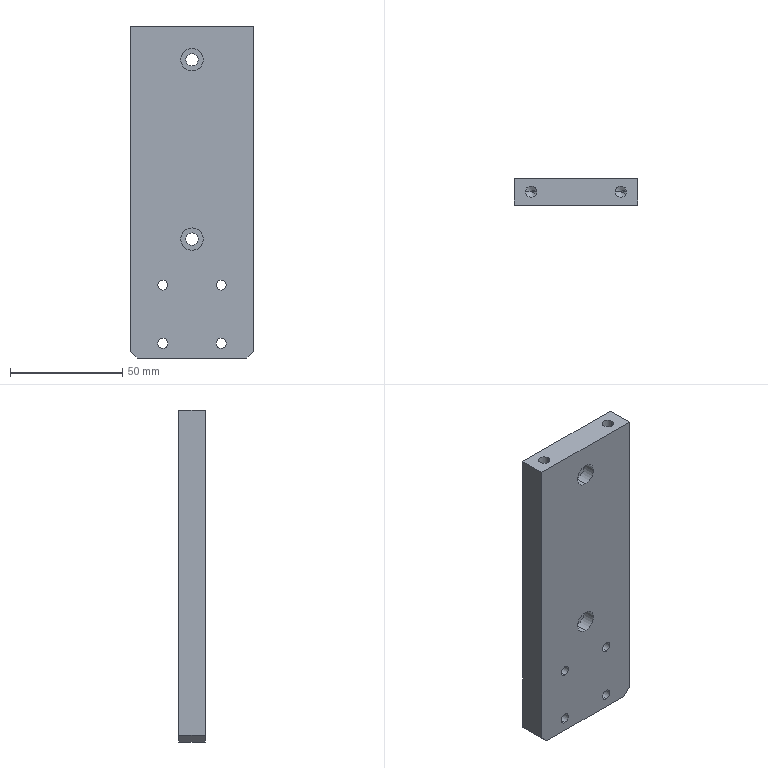Part | SolidWorks | features HoleWzd 3, Chamfer 1, Extrusion 1 | 1 solid | 46 faces | box 55 x 12 x 148 mm | volume 94373 mm3 | cylinder 28 | plane 14 | cone 4 | commonest cylinder face diameters 4.5 x8 8 x8 5 x4 5.5 x4 10 x4
STEP:
#1=CARTESIAN_POINT('',(0.,-0.3,64.));
#2=VERTEX_POINT('',#1);
#3=CARTESIAN_POINT('',(0.,-0.3,54.));
#4=VERTEX_POINT('',#3);
#5=CARTESIAN_POINT('',(0.,-0.3,59.));
#6=DIRECTION('',(0.,-1.,0.));
#7=DIRECTION('',(0.,0.,-1.));
#8=AXIS2_PLACEMENT_3D('',#5,#6,#7);
#9=CIRCLE('',#8,5.);
#10=EDGE_CURVE('',#2,#4,#9,.T.);
#11=ORIENTED_EDGE('',*,*,#10,.F.);
#12=CARTESIAN_POINT('',(0.,-6.,64.));
#13=VERTEX_POINT('',#12);
#14=CARTESIAN_POINT('',(0.,-6.,64.));
#15=DIRECTION('',(0.,-1.,0.));
#16=VECTOR('',#15,1000.);
#17=LINE('',#14,#16);
#18=EDGE_CURVE('',#2,#13,#17,.T.);
#19=ORIENTED_EDGE('',*,*,#18,.T.);
#20=CARTESIAN_POINT('',(0.,-6.,54.));
#21=VERTEX_POINT('',#20);
#22=CARTESIAN_POINT('',(0.,-6.,59.));
#23=DIRECTION('',(0.,-1.,0.));
#24=DIRECTION('',(0.,0.,-1.));
#25=AXIS2_PLACEMENT_3D('',#22,#23,#24);
#26=CIRCLE('',#25,5.);
#27=EDGE_CURVE('',#13,#21,#26,.T.);
#28=ORIENTED_EDGE('',*,*,#27,.T.);
#29=CARTESIAN_POINT('',(0.,-6.,54.));
#30=DIRECTION('',(0.,-1.,0.));
#31=VECTOR('',#30,1000.);
#32=LINE('',#29,#31);
#33=EDGE_CURVE('',#4,#21,#32,.T.);
#34=ORIENTED_EDGE('',*,*,#33,.F.);
#35=EDGE_LOOP('',(#11,#19,#28,#34));
#36=FACE_OUTER_BOUND('',#35,.T.);
#37=CARTESIAN_POINT('',(0.,-6.,59.));
#38=DIRECTION('',(0.,-1.,0.));
#39=DIRECTION('',(0.,0.,-1.));
#40=AXIS2_PLACEMENT_3D('',#37,#38,#39);
#41=CYLINDRICAL_SURFACE('',#40,5.);
#42=ADVANCED_FACE('',(#36),#41,.F.);
#43=CARTESIAN_POINT('',(0.,6.,61.75));
#44=VERTEX_POINT('',#43);
#45=CARTESIAN_POINT('',(0.,6.,56.25));
#46=VERTEX_POINT('',#45);
#47=CARTESIAN_POINT('',(0.,6.,59.));
#48=DIRECTION('',(0.,-1.,0.));
#49=DIRECTION('',(0.,0.,-1.));
#50=AXIS2_PLACEMENT_3D('',#47,#48,#49);
#51=CIRCLE('',#50,2.75);
#52=EDGE_CURVE('',#44,#46,#51,.T.);
#53=ORIENTED_EDGE('',*,*,#52,.F.);
#54=CARTESIAN_POINT('',(0.,-0.3,61.75));
#55=VERTEX_POINT('',#54);
#56=CARTESIAN_POINT('',(0.,-6.,61.75));
#57=DIRECTION('',(0.,-1.,0.));
#58=VECTOR('',#57,1000.);
#59=LINE('',#56,#58);
#60=EDGE_CURVE('',#44,#55,#59,.T.);
#61=ORIENTED_EDGE('',*,*,#60,.T.);
#62=CARTESIAN_POINT('',(0.,-0.3,56.25));
#63=VERTEX_POINT('',#62);
#64=CARTESIAN_POINT('',(0.,-0.3,59.));
#65=DIRECTION('',(0.,-1.,0.));
#66=DIRECTION('',(0.,0.,-1.));
#67=AXIS2_PLACEMENT_3D('',#64,#65,#66);
#68=CIRCLE('',#67,2.75);
#69=EDGE_CURVE('',#55,#63,#68,.T.);
#70=ORIENTED_EDGE('',*,*,#69,.T.);
#71=CARTESIAN_POINT('',(0.,-6.,56.25));
#72=DIRECTION('',(0.,-1.,0.));
#73=VECTOR('',#72,1000.);
#74=LINE('',#71,#73);
#75=EDGE_CURVE('',#46,#63,#74,.T.);
#76=ORIENTED_EDGE('',*,*,#75,.F.);
#77=EDGE_LOOP('',(#53,#61,#70,#76));
#78=FACE_OUTER_BOUND('',#77,.T.);
#79=CARTESIAN_POINT('',(0.,-6.,59.));
#80=DIRECTION('',(0.,-1.,0.));
#81=DIRECTION('',(0.,0.,-1.));
#82=AXIS2_PLACEMENT_3D('',#79,#80,#81);
#83=CYLINDRICAL_SURFACE('',#82,2.75);
#84=ADVANCED_FACE('',(#78),#83,.F.);
#85=CARTESIAN_POINT('',(0.,-0.3,-16.));
#86=VERTEX_POINT('',#85);
#87=CARTESIAN_POINT('',(0.,-0.3,-26.));
#88=VERTEX_POINT('',#87);
#89=CARTESIAN_POINT('',(0.,-0.3,-21.));
#90=DIRECTION('',(0.,-1.,0.));
#91=DIRECTION('',(0.,0.,-1.));
#92=AXIS2_PLACEMENT_3D('',#89,#90,#91);
#93=CIRCLE('',#92,5.);
#94=EDGE_CURVE('',#86,#88,#93,.T.);
#95=ORIENTED_EDGE('',*,*,#94,.F.);
#96=CARTESIAN_POINT('',(0.,-6.,-16.));
#97=VERTEX_POINT('',#96);
#98=CARTESIAN_POINT('',(0.,-6.,-16.));
#99=DIRECTION('',(0.,-1.,0.));
#100=VECTOR('',#99,1000.);
#101=LINE('',#98,#100);
#102=EDGE_CURVE('',#86,#97,#101,.T.);
#103=ORIENTED_EDGE('',*,*,#102,.T.);
#104=CARTESIAN_POINT('',(0.,-6.,-26.));
#105=VERTEX_POINT('',#104);
#106=CARTESIAN_POINT('',(0.,-6.,-21.));
#107=DIRECTION('',(0.,-1.,0.));
#108=DIRECTION('',(0.,0.,-1.));
#109=AXIS2_PLACEMENT_3D('',#106,#107,#108);
#110=CIRCLE('',#109,5.);
#111=EDGE_CURVE('',#97,#105,#110,.T.);
#112=ORIENTED_EDGE('',*,*,#111,.T.);
#113=CARTESIAN_POINT('',(0.,-6.,-26.));
#114=DIRECTION('',(0.,-1.,0.));
#115=VECTOR('',#114,1000.);
#116=LINE('',#113,#115);
#117=EDGE_CURVE('',#88,#105,#116,.T.);
#118=ORIENTED_EDGE('',*,*,#117,.F.);
#119=EDGE_LOOP('',(#95,#103,#112,#118));
#120=FACE_OUTER_BOUND('',#119,.T.);
#121=CARTESIAN_POINT('',(0.,-6.,-21.));
#122=DIRECTION('',(0.,-1.,0.));
#123=DIRECTION('',(0.,0.,-1.));
#124=AXIS2_PLACEMENT_3D('',#121,#122,#123);
#125=CYLINDRICAL_SURFACE('',#124,5.);
#126=ADVANCED_FACE('',(#120),#125,.F.);
#127=CARTESIAN_POINT('',(0.,6.,-18.25));
#128=VERTEX_POINT('',#127);
#129=CARTESIAN_POINT('',(0.,6.,-23.75));
#130=VERTEX_POINT('',#129);
#131=CARTESIAN_POINT('',(0.,6.,-21.));
#132=DIRECTION('',(0.,-1.,0.));
#133=DIRECTION('',(0.,0.,-1.));
#134=AXIS2_PLACEMENT_3D('',#131,#132,#133);
#135=CIRCLE('',#134,2.75);
#136=EDGE_CURVE('',#128,#130,#135,.T.);
#137=ORIENTED_EDGE('',*,*,#136,.F.);
#138=CARTESIAN_POINT('',(0.,-0.3,-18.25));
#139=VERTEX_POINT('',#138);
#140=CARTESIAN_POINT('',(0.,-6.,-18.25));
#141=DIRECTION('',(0.,-1.,0.));
#142=VECTOR('',#141,1000.);
#143=LINE('',#140,#142);
#144=EDGE_CURVE('',#128,#139,#143,.T.);
#145=ORIENTED_EDGE('',*,*,#144,.T.);
#146=CARTESIAN_POINT('',(0.,-0.3,-23.75));
#147=VERTEX_POINT('',#146);
#148=CARTESIAN_POINT('',(0.,-0.3,-21.));
#149=DIRECTION('',(0.,-1.,0.));
#150=DIRECTION('',(0.,0.,-1.));
#151=AXIS2_PLACEMENT_3D('',#148,#149,#150);
#152=CIRCLE('',#151,2.75);
#153=EDGE_CURVE('',#139,#147,#152,.T.);
#154=ORIENTED_EDGE('',*,*,#153,.T.);
#155=CARTESIAN_POINT('',(0.,-6.,-23.75));
#156=DIRECTION('',(0.,-1.,0.));
#157=VECTOR('',#156,1000.);
#158=LINE('',#155,#157);
#159=EDGE_CURVE('',#130,#147,#158,.T.);
#160=ORIENTED_EDGE('',*,*,#159,.F.);
#161=EDGE_LOOP('',(#137,#145,#154,#160));
#162=FACE_OUTER_BOUND('',#161,.T.);
#163=CARTESIAN_POINT('',(0.,-6.,-21.));
#164=DIRECTION('',(0.,-1.,0.));
#165=DIRECTION('',(0.,0.,-1.));
#166=AXIS2_PLACEMENT_3D('',#163,#164,#165);
#167=CYLINDRICAL_SURFACE('',#166,2.75);
#168=ADVANCED_FACE('',(#162),#167,.F.);
#169=CARTESIAN_POINT('',(17.5,0.,59.));
#170=VERTEX_POINT('',#169);
#171=CARTESIAN_POINT('',(22.5,0.,59.));
#172=VERTEX_POINT('',#171);
#173=CARTESIAN_POINT('',(20.,0.,59.));
#174=DIRECTION('',(0.,0.,1.));
#175=DIRECTION('',(1.,0.,0.));
#176=AXIS2_PLACEMENT_3D('',#173,#174,#175);
#177=CIRCLE('',#176,2.5);
#178=EDGE_CURVE('',#170,#172,#177,.T.);
#179=ORIENTED_EDGE('',*,*,#178,.F.);
#180=CARTESIAN_POINT('',(17.5,0.,74.));
#181=VERTEX_POINT('',#180);
#182=CARTESIAN_POINT('',(17.5,0.,74.));
#183=DIRECTION('',(0.,0.,1.));
#184=VECTOR('',#183,1000.);
#185=LINE('',#182,#184);
#186=EDGE_CURVE('',#170,#181,#185,.T.);
#187=ORIENTED_EDGE('',*,*,#186,.T.);
#188=CARTESIAN_POINT('',(22.5,0.,74.));
#189=VERTEX_POINT('',#188);
#190=CARTESIAN_POINT('',(20.,0.,74.));
#191=DIRECTION('',(0.,0.,1.));
#192=DIRECTION('',(1.,0.,0.));
#193=AXIS2_PLACEMENT_3D('',#190,#191,#192);
#194=CIRCLE('',#193,2.5);
#195=EDGE_CURVE('',#181,#189,#194,.T.);
#196=ORIENTED_EDGE('',*,*,#195,.T.);
#197=CARTESIAN_POINT('',(22.5,0.,74.));
#198=DIRECTION('',(0.,0.,1.));
#199=VECTOR('',#198,1000.);
#200=LINE('',#197,#199);
#201=EDGE_CURVE('',#172,#189,#200,.T.);
#202=ORIENTED_EDGE('',*,*,#201,.F.);
#203=EDGE_LOOP('',(#179,#187,#196,#202));
#204=FACE_OUTER_BOUND('',#203,.T.);
#205=CARTESIAN_POINT('',(20.,0.,74.));
#206=DIRECTION('',(0.,0.,1.));
#207=DIRECTION('',(1.,0.,0.));
#208=AXIS2_PLACEMENT_3D('',#205,#206,#207);
#209=CYLINDRICAL_SURFACE('',#208,2.5);
#210=ADVANCED_FACE('',(#204),#209,.F.);
#211=CARTESIAN_POINT('',(20.,0.,57.498));
#212=VERTEX_POINT('',#211);
#213=CARTESIAN_POINT('',(22.5,0.,59.));
#214=DIRECTION('',(0.8572,0.,0.515));
#215=VECTOR('',#214,1000.);
#216=LINE('',#213,#215);
#217=EDGE_CURVE('',#212,#172,#216,.T.);
#218=ORIENTED_EDGE('',*,*,#217,.F.);
#219=CARTESIAN_POINT('',(17.5,0.,59.));
#220=DIRECTION('',(-0.8572,0.,0.515));
#221=VECTOR('',#220,1000.);
#222=LINE('',#219,#221);
#223=EDGE_CURVE('',#212,#170,#222,.T.);
#224=ORIENTED_EDGE('',*,*,#223,.T.);
#225=ORIENTED_EDGE('',*,*,#178,.T.);
#226=EDGE_LOOP('',(#218,#224,#225));
#227=FACE_OUTER_BOUND('',#226,.T.);
#228=CARTESIAN_POINT('',(20.,0.,59.));
#229=DIRECTION('',(0.,0.,1.));
#230=DIRECTION('',(1.,0.,0.));
#231=AXIS2_PLACEMENT_3D('',#228,#229,#230);
#232=CONICAL_SURFACE('',#231,2.5,1.03);
#233=ADVANCED_FACE('',(#227),#232,.F.);
#234=CARTESIAN_POINT('',(-22.5,0.,59.));
#235=VERTEX_POINT('',#234);
#236=CARTESIAN_POINT('',(-17.5,0.,59.));
#237=VERTEX_POINT('',#236);
#238=CARTESIAN_POINT('',(-20.,0.,59.));
#239=DIRECTION('',(0.,0.,1.));
#240=DIRECTION('',(1.,0.,0.));
#241=AXIS2_PLACEMENT_3D('',#238,#239,#240);
#242=CIRCLE('',#241,2.5);
#243=EDGE_CURVE('',#235,#237,#242,.T.);
#244=ORIENTED_EDGE('',*,*,#243,.F.);
#245=CARTESIAN_POINT('',(-22.5,0.,74.));
#246=VERTEX_POINT('',#245);
#247=CARTESIAN_POINT('',(-22.5,0.,74.));
#248=DIRECTION('',(0.,0.,1.));
#249=VECTOR('',#248,1000.);
#250=LINE('',#247,#249);
#251=EDGE_CURVE('',#235,#246,#250,.T.);
#252=ORIENTED_EDGE('',*,*,#251,.T.);
#253=CARTESIAN_POINT('',(-17.5,0.,74.));
#254=VERTEX_POINT('',#253);
#255=CARTESIAN_POINT('',(-20.,0.,74.));
#256=DIRECTION('',(0.,0.,1.));
#257=DIRECTION('',(1.,0.,0.));
#258=AXIS2_PLACEMENT_3D('',#255,#256,#257);
#259=CIRCLE('',#258,2.5);
#260=EDGE_CURVE('',#246,#254,#259,.T.);
#261=ORIENTED_EDGE('',*,*,#260,.T.);
#262=CARTESIAN_POINT('',(-17.5,0.,74.));
#263=DIRECTION('',(0.,0.,1.));
#264=VECTOR('',#263,1000.);
#265=LINE('',#262,#264);
#266=EDGE_CURVE('',#237,#254,#265,.T.);
#267=ORIENTED_EDGE('',*,*,#266,.F.);
#268=EDGE_LOOP('',(#244,#252,#261,#267));
#269=FACE_OUTER_BOUND('',#268,.T.);
#270=CARTESIAN_POINT('',(-20.,0.,74.));
#271=DIRECTION('',(0.,0.,1.));
#272=DIRECTION('',(1.,0.,0.));
#273=AXIS2_PLACEMENT_3D('',#270,#271,#272);
#274=CYLINDRICAL_SURFACE('',#273,2.5);
#275=ADVANCED_FACE('',(#269),#274,.F.);
#276=CARTESIAN_POINT('',(-20.,0.,57.498));
#277=VERTEX_POINT('',#276);
#278=CARTESIAN_POINT('',(-17.5,0.,59.));
#279=DIRECTION('',(0.8572,0.,0.515));
#280=VECTOR('',#279,1000.);
#281=LINE('',#278,#280);
#282=EDGE_CURVE('',#277,#237,#281,.T.);
#283=ORIENTED_EDGE('',*,*,#282,.F.);
#284=CARTESIAN_POINT('',(-22.5,0.,59.));
#285=DIRECTION('',(-0.8572,0.,0.515));
#286=VECTOR('',#285,1000.);
#287=LINE('',#284,#286);
#288=EDGE_CURVE('',#277,#235,#287,.T.);
#289=ORIENTED_EDGE('',*,*,#288,.T.);
#290=ORIENTED_EDGE('',*,*,#243,.T.);
#291=EDGE_LOOP('',(#283,#289,#290));
#292=FACE_OUTER_BOUND('',#291,.T.);
#293=CARTESIAN_POINT('',(-20.,0.,59.));
#294=DIRECTION('',(0.,0.,1.));
#295=DIRECTION('',(1.,0.,0.));
#296=AXIS2_PLACEMENT_3D('',#293,#294,#295);
#297=CONICAL_SURFACE('',#296,2.5,1.03);
#298=ADVANCED_FACE('',(#292),#297,.F.);
#299=CARTESIAN_POINT('',(13.,1.4,-45.5));
#300=VERTEX_POINT('',#299);
#301=CARTESIAN_POINT('',(13.,1.4,-37.5));
#302=VERTEX_POINT('',#301);
#303=CARTESIAN_POINT('',(13.,1.4,-41.5));
#304=DIRECTION('',(0.,1.,0.));
#305=DIRECTION('',(0.,0.,1.));
#306=AXIS2_PLACEMENT_3D('',#303,#304,#305);
#307=CIRCLE('',#306,4.);
#308=EDGE_CURVE('',#300,#302,#307,.T.);
#309=ORIENTED_EDGE('',*,*,#308,.F.);
#310=CARTESIAN_POINT('',(13.,6.,-45.5));
#311=VERTEX_POINT('',#310);
#312=CARTESIAN_POINT('',(13.,6.,-45.5));
#313=DIRECTION('',(0.,1.,0.));
#314=VECTOR('',#313,1000.);
#315=LINE('',#312,#314);
#316=EDGE_CURVE('',#300,#311,#315,.T.);
#317=ORIENTED_EDGE('',*,*,#316,.T.);
#318=CARTESIAN_POINT('',(13.,6.,-37.5));
#319=VERTEX_POINT('',#318);
#320=CARTESIAN_POINT('',(13.,6.,-41.5));
#321=DIRECTION('',(0.,1.,0.));
#322=DIRECTION('',(0.,0.,1.));
#323=AXIS2_PLACEMENT_3D('',#320,#321,#322);
#324=CIRCLE('',#323,4.);
#325=EDGE_CURVE('',#311,#319,#324,.T.);
#326=ORIENTED_EDGE('',*,*,#325,.T.);
#327=CARTESIAN_POINT('',(13.,6.,-37.5));
#328=DIRECTION('',(0.,1.,0.));
#329=VECTOR('',#328,1000.);
#330=LINE('',#327,#329);
#331=EDGE_CURVE('',#302,#319,#330,.T.);
#332=ORIENTED_EDGE('',*,*,#331,.F.);
#333=EDGE_LOOP('',(#309,#317,#326,#332));
#334=FACE_OUTER_BOUND('',#333,.T.);
#335=CARTESIAN_POINT('',(13.,6.,-41.5));
#336=DIRECTION('',(0.,1.,0.));
#337=DIRECTION('',(0.,0.,1.));
#338=AXIS2_PLACEMENT_3D('',#335,#336,#337);
#339=CYLINDRICAL_SURFACE('',#338,4.);
#340=ADVANCED_FACE('',(#334),#339,.F.);
#341=CARTESIAN_POINT('',(13.,-6.,-43.75));
#342=VERTEX_POINT('',#341);
#343=CARTESIAN_POINT('',(13.,-6.,-39.25));
#344=VERTEX_POINT('',#343);
#345=CARTESIAN_POINT('',(13.,-6.,-41.5));
#346=DIRECTION('',(0.,1.,0.));
#347=DIRECTION('',(0.,0.,1.));
#348=AXIS2_PLACEMENT_3D('',#345,#346,#347);
#349=CIRCLE('',#348,2.25);
#350=EDGE_CURVE('',#342,#344,#349,.T.);
#351=ORIENTED_EDGE('',*,*,#350,.F.);
#352=CARTESIAN_POINT('',(13.,1.4,-43.75));
#353=VERTEX_POINT('',#352);
#354=CARTESIAN_POINT('',(13.,6.,-43.75));
#355=DIRECTION('',(0.,1.,0.));
#356=VECTOR('',#355,1000.);
#357=LINE('',#354,#356);
#358=EDGE_CURVE('',#342,#353,#357,.T.);
#359=ORIENTED_EDGE('',*,*,#358,.T.);
#360=CARTESIAN_POINT('',(13.,1.4,-39.25));
#361=VERTEX_POINT('',#360);
#362=CARTESIAN_POINT('',(13.,1.4,-41.5));
#363=DIRECTION('',(0.,1.,0.));
#364=DIRECTION('',(0.,0.,1.));
#365=AXIS2_PLACEMENT_3D('',#362,#363,#364);
#366=CIRCLE('',#365,2.25);
#367=EDGE_CURVE('',#353,#361,#366,.T.);
#368=ORIENTED_EDGE('',*,*,#367,.T.);
#369=CARTESIAN_POINT('',(13.,6.,-39.25));
#370=DIRECTION('',(0.,1.,0.));
#371=VECTOR('',#370,1000.);
#372=LINE('',#369,#371);
#373=EDGE_CURVE('',#344,#361,#372,.T.);
#374=ORIENTED_EDGE('',*,*,#373,.F.);
#375=EDGE_LOOP('',(#351,#359,#368,#374));
#376=FACE_OUTER_BOUND('',#375,.T.);
#377=CARTESIAN_POINT('',(13.,6.,-41.5));
#378=DIRECTION('',(0.,1.,0.));
#379=DIRECTION('',(0.,0.,1.));
#380=AXIS2_PLACEMENT_3D('',#377,#378,#379);
#381=CYLINDRICAL_SURFACE('',#380,2.25);
#382=ADVANCED_FACE('',(#376),#381,.F.);
#383=CARTESIAN_POINT('',(13.,1.4,-71.5));
#384=VERTEX_POINT('',#383);
#385=CARTESIAN_POINT('',(13.,1.4,-63.5));
#386=VERTEX_POINT('',#385);
#387=CARTESIAN_POINT('',(13.,1.4,-67.5));
#388=DIRECTION('',(0.,1.,0.));
#389=DIRECTION('',(0.,0.,1.));
#390=AXIS2_PLACEMENT_3D('',#387,#388,#389);
#391=CIRCLE('',#390,4.);
#392=EDGE_CURVE('',#384,#386,#391,.T.);
#393=ORIENTED_EDGE('',*,*,#392,.F.);
#394=CARTESIAN_POINT('',(13.,6.,-71.5));
#395=VERTEX_POINT('',#394);
#396=CARTESIAN_POINT('',(13.,6.,-71.5));
#397=DIRECTION('',(0.,1.,0.));
#398=VECTOR('',#397,1000.);
#399=LINE('',#396,#398);
#400=EDGE_CURVE('',#384,#395,#399,.T.);
#401=ORIENTED_EDGE('',*,*,#400,.T.);
#402=CARTESIAN_POINT('',(13.,6.,-63.5));
#403=VERTEX_POINT('',#402);
#404=CARTESIAN_POINT('',(13.,6.,-67.5));
#405=DIRECTION('',(0.,1.,0.));
#406=DIRECTION('',(0.,0.,1.));
#407=AXIS2_PLACEMENT_3D('',#404,#405,#406);
#408=CIRCLE('',#407,4.);
#409=EDGE_CURVE('',#395,#403,#408,.T.);
#410=ORIENTED_EDGE('',*,*,#409,.T.);
#411=CARTESIAN_POINT('',(13.,6.,-63.5));
#412=DIRECTION('',(0.,1.,0.));
#413=VECTOR('',#412,1000.);
#414=LINE('',#411,#413);
#415=EDGE_CURVE('',#386,#403,#414,.T.);
#416=ORIENTED_EDGE('',*,*,#415,.F.);
#417=EDGE_LOOP('',(#393,#401,#410,#416));
#418=FACE_OUTER_BOUND('',#417,.T.);
#419=CARTESIAN_POINT('',(13.,6.,-67.5));
#420=DIRECTION('',(0.,1.,0.));
#421=DIRECTION('',(0.,0.,1.));
#422=AXIS2_PLACEMENT_3D('',#419,#420,#421);
#423=CYLINDRICAL_SURFACE('',#422,4.);
#424=ADVANCED_FACE('',(#418),#423,.F.);
#425=CARTESIAN_POINT('',(13.,-6.,-69.75));
#426=VERTEX_POINT('',#425);
#427=CARTESIAN_POINT('',(13.,-6.,-65.25));
#428=VERTEX_POINT('',#427);
#429=CARTESIAN_POINT('',(13.,-6.,-67.5));
#430=DIRECTION('',(0.,1.,0.));
#431=DIRECTION('',(0.,0.,1.));
#432=AXIS2_PLACEMENT_3D('',#429,#430,#431);
#433=CIRCLE('',#432,2.25);
#434=EDGE_CURVE('',#426,#428,#433,.T.);
#435=ORIENTED_EDGE('',*,*,#434,.F.);
#436=CARTESIAN_POINT('',(13.,1.4,-69.75));
#437=VERTEX_POINT('',#436);
#438=CARTESIAN_POINT('',(13.,6.,-69.75));
#439=DIRECTION('',(0.,1.,0.));
#440=VECTOR('',#439,1000.);
#441=LINE('',#438,#440);
#442=EDGE_CURVE('',#426,#437,#441,.T.);
#443=ORIENTED_EDGE('',*,*,#442,.T.);
#444=CARTESIAN_POINT('',(13.,1.4,-65.25));
#445=VERTEX_POINT('',#444);
#446=CARTESIAN_POINT('',(13.,1.4,-67.5));
#447=DIRECTION('',(0.,1.,0.));
#448=DIRECTION('',(0.,0.,1.));
#449=AXIS2_PLACEMENT_3D('',#446,#447,#448);
#450=CIRCLE('',#449,2.25);
#451=EDGE_CURVE('',#437,#445,#450,.T.);
#452=ORIENTED_EDGE('',*,*,#451,.T.);
#453=CARTESIAN_POINT('',(13.,6.,-65.25));
#454=DIRECTION('',(0.,1.,0.));
#455=VECTOR('',#454,1000.);
#456=LINE('',#453,#455);
#457=EDGE_CURVE('',#428,#445,#456,.T.);
#458=ORIENTED_EDGE('',*,*,#457,.F.);
#459=EDGE_LOOP('',(#435,#443,#452,#458));
#460=FACE_OUTER_BOUND('',#459,.T.);
#461=CARTESIAN_POINT('',(13.,6.,-67.5));
#462=DIRECTION('',(0.,1.,0.));
#463=DIRECTION('',(0.,0.,1.));
#464=AXIS2_PLACEMENT_3D('',#461,#462,#463);
#465=CYLINDRICAL_SURFACE('',#464,2.25);
#466=ADVANCED_FACE('',(#460),#465,.F.);
#467=CARTESIAN_POINT('',(-13.,1.4,-71.5));
#468=VERTEX_POINT('',#467);
#469=CARTESIAN_POINT('',(-13.,1.4,-63.5));
#470=VERTEX_POINT('',#469);
#471=CARTESIAN_POINT('',(-13.,1.4,-67.5));
#472=DIRECTION('',(0.,1.,0.));
#473=DIRECTION('',(0.,0.,1.));
#474=AXIS2_PLACEMENT_3D('',#471,#472,#473);
#475=CIRCLE('',#474,4.);
#476=EDGE_CURVE('',#468,#470,#475,.T.);
#477=ORIENTED_EDGE('',*,*,#476,.F.);
#478=CARTESIAN_POINT('',(-13.,6.,-71.5));
#479=VERTEX_POINT('',#478);
#480=CARTESIAN_POINT('',(-13.,6.,-71.5));
#481=DIRECTION('',(0.,1.,0.));
#482=VECTOR('',#481,1000.);
#483=LINE('',#480,#482);
#484=EDGE_CURVE('',#468,#479,#483,.T.);
#485=ORIENTED_EDGE('',*,*,#484,.T.);
#486=CARTESIAN_POINT('',(-13.,6.,-63.5));
#487=VERTEX_POINT('',#486);
#488=CARTESIAN_POINT('',(-13.,6.,-67.5));
#489=DIRECTION('',(0.,1.,0.));
#490=DIRECTION('',(0.,0.,1.));
#491=AXIS2_PLACEMENT_3D('',#488,#489,#490);
#492=CIRCLE('',#491,4.);
#493=EDGE_CURVE('',#479,#487,#492,.T.);
#494=ORIENTED_EDGE('',*,*,#493,.T.);
#495=CARTESIAN_POINT('',(-13.,6.,-63.5));
#496=DIRECTION('',(0.,1.,0.));
#497=VECTOR('',#496,1000.);
#498=LINE('',#495,#497);
#499=EDGE_CURVE('',#470,#487,#498,.T.);
#500=ORIENTED_EDGE('',*,*,#499,.F.);
#501=EDGE_LOOP('',(#477,#485,#494,#500));
#502=FACE_OUTER_BOUND('',#501,.T.);
#503=CARTESIAN_POINT('',(-13.,6.,-67.5));
#504=DIRECTION('',(0.,1.,0.));
#505=DIRECTION('',(0.,0.,1.));
#506=AXIS2_PLACEMENT_3D('',#503,#504,#505);
#507=CYLINDRICAL_SURFACE('',#506,4.);
#508=ADVANCED_FACE('',(#502),#507,.F.);
#509=CARTESIAN_POINT('',(-13.,-6.,-69.75));
#510=VERTEX_POINT('',#509);
#511=CARTESIAN_POINT('',(-13.,-6.,-65.25));
#512=VERTEX_POINT('',#511);
#513=CARTESIAN_POINT('',(-13.,-6.,-67.5));
#514=DIRECTION('',(0.,1.,0.));
#515=DIRECTION('',(0.,0.,1.));
#516=AXIS2_PLACEMENT_3D('',#513,#514,#515);
#517=CIRCLE('',#516,2.25);
#518=EDGE_CURVE('',#510,#512,#517,.T.);
#519=ORIENTED_EDGE('',*,*,#518,.F.);
#520=CARTESIAN_POINT('',(-13.,1.4,-69.75));
#521=VERTEX_POINT('',#520);
#522=CARTESIAN_POINT('',(-13.,6.,-69.75));
#523=DIRECTION('',(0.,1.,0.));
#524=VECTOR('',#523,1000.);
#525=LINE('',#522,#524);
#526=EDGE_CURVE('',#510,#521,#525,.T.);
#527=ORIENTED_EDGE('',*,*,#526,.T.);
#528=CARTESIAN_POINT('',(-13.,1.4,-65.25));
#529=VERTEX_POINT('',#528);
#530=CARTESIAN_POINT('',(-13.,1.4,-67.5));
#531=DIRECTION('',(0.,1.,0.));
#532=DIRECTION('',(0.,0.,1.));
#533=AXIS2_PLACEMENT_3D('',#530,#531,#532);
#534=CIRCLE('',#533,2.25);
#535=EDGE_CURVE('',#521,#529,#534,.T.);
#536=ORIENTED_EDGE('',*,*,#535,.T.);
#537=CARTESIAN_POINT('',(-13.,6.,-65.25));
#538=DIRECTION('',(0.,1.,0.));
#539=VECTOR('',#538,1000.);
#540=LINE('',#537,#539);
#541=EDGE_CURVE('',#512,#529,#540,.T.);
#542=ORIENTED_EDGE('',*,*,#541,.F.);
#543=EDGE_LOOP('',(#519,#527,#536,#542));
#544=FACE_OUTER_BOUND('',#543,.T.);
#545=CARTESIAN_POINT('',(-13.,6.,-67.5));
#546=DIRECTION('',(0.,1.,0.));
#547=DIRECTION('',(0.,0.,1.));
#548=AXIS2_PLACEMENT_3D('',#545,#546,#547);
#549=CYLINDRICAL_SURFACE('',#548,2.25);
#550=ADVANCED_FACE('',(#544),#549,.F.);
#551=CARTESIAN_POINT('',(-13.,1.4,-45.5));
#552=VERTEX_POINT('',#551);
#553=CARTESIAN_POINT('',(-13.,1.4,-37.5));
#554=VERTEX_POINT('',#553);
#555=CARTESIAN_POINT('',(-13.,1.4,-41.5));
#556=DIRECTION('',(0.,1.,0.));
#557=DIRECTION('',(0.,0.,1.));
#558=AXIS2_PLACEMENT_3D('',#555,#556,#557);
#559=CIRCLE('',#558,4.);
#560=EDGE_CURVE('',#552,#554,#559,.T.);
#561=ORIENTED_EDGE('',*,*,#560,.F.);
#562=CARTESIAN_POINT('',(-13.,6.,-45.5));
#563=VERTEX_POINT('',#562);
#564=CARTESIAN_POINT('',(-13.,6.,-45.5));
#565=DIRECTION('',(0.,1.,0.));
#566=VECTOR('',#565,1000.);
#567=LINE('',#564,#566);
#568=EDGE_CURVE('',#552,#563,#567,.T.);
#569=ORIENTED_EDGE('',*,*,#568,.T.);
#570=CARTESIAN_POINT('',(-13.,6.,-37.5));
#571=VERTEX_POINT('',#570);
#572=CARTESIAN_POINT('',(-13.,6.,-41.5));
#573=DIRECTION('',(0.,1.,0.));
#574=DIRECTION('',(0.,0.,1.));
#575=AXIS2_PLACEMENT_3D('',#572,#573,#574);
#576=CIRCLE('',#575,4.);
#577=EDGE_CURVE('',#563,#571,#576,.T.);
#578=ORIENTED_EDGE('',*,*,#577,.T.);
#579=CARTESIAN_POINT('',(-13.,6.,-37.5));
#580=DIRECTION('',(0.,1.,0.));
#581=VECTOR('',#580,1000.);
#582=LINE('',#579,#581);
#583=EDGE_CURVE('',#554,#571,#582,.T.);
#584=ORIENTED_EDGE('',*,*,#583,.F.);
#585=EDGE_LOOP('',(#561,#569,#578,#584));
#586=FACE_OUTER_BOUND('',#585,.T.);
#587=CARTESIAN_POINT('',(-13.,6.,-41.5));
#588=DIRECTION('',(0.,1.,0.));
#589=DIRECTION('',(0.,0.,1.));
#590=AXIS2_PLACEMENT_3D('',#587,#588,#589);
#591=CYLINDRICAL_SURFACE('',#590,4.);
#592=ADVANCED_FACE('',(#586),#591,.F.);
#593=CARTESIAN_POINT('',(-13.,-6.,-43.75));
#594=VERTEX_POINT('',#593);
#595=CARTESIAN_POINT('',(-13.,-6.,-39.25));
#596=VERTEX_POINT('',#595);
#597=CARTESIAN_POINT('',(-13.,-6.,-41.5));
#598=DIRECTION('',(0.,1.,0.));
#599=DIRECTION('',(0.,0.,1.));
#600=AXIS2_PLACEMENT_3D('',#597,#598,#599);
#601=CIRCLE('',#600,2.25);
#602=EDGE_CURVE('',#594,#596,#601,.T.);
#603=ORIENTED_EDGE('',*,*,#602,.F.);
#604=CARTESIAN_POINT('',(-13.,1.4,-43.75));
#605=VERTEX_POINT('',#604);
#606=CARTESIAN_POINT('',(-13.,6.,-43.75));
#607=DIRECTION('',(0.,1.,0.));
#608=VECTOR('',#607,1000.);
#609=LINE('',#606,#608);
#610=EDGE_CURVE('',#594,#605,#609,.T.);
#611=ORIENTED_EDGE('',*,*,#610,.T.);
#612=CARTESIAN_POINT('',(-13.,1.4,-39.25));
#613=VERTEX_POINT('',#612);
#614=CARTESIAN_POINT('',(-13.,1.4,-41.5));
#615=DIRECTION('',(0.,1.,0.));
#616=DIRECTION('',(0.,0.,1.));
#617=AXIS2_PLACEMENT_3D('',#614,#615,#616);
#618=CIRCLE('',#617,2.25);
#619=EDGE_CURVE('',#605,#613,#618,.T.);
#620=ORIENTED_EDGE('',*,*,#619,.T.);
#621=CARTESIAN_POINT('',(-13.,6.,-39.25));
#622=DIRECTION('',(0.,1.,0.));
#623=VECTOR('',#622,1000.);
#624=LINE('',#621,#623);
#625=EDGE_CURVE('',#596,#613,#624,.T.);
#626=ORIENTED_EDGE('',*,*,#625,.F.);
#627=EDGE_LOOP('',(#603,#611,#620,#626));
#628=FACE_OUTER_BOUND('',#627,.T.);
#629=CARTESIAN_POINT('',(-13.,6.,-41.5));
#630=DIRECTION('',(0.,1.,0.));
#631=DIRECTION('',(0.,0.,1.));
#632=AXIS2_PLACEMENT_3D('',#629,#630,#631);
#633=CYLINDRICAL_SURFACE('',#632,2.25);
#634=ADVANCED_FACE('',(#628),#633,.F.);
#635=CARTESIAN_POINT('',(27.5,-6.,74.));
#636=VERTEX_POINT('',#635);
#637=CARTESIAN_POINT('',(27.5,-6.,-71.));
#638=VERTEX_POINT('',#637);
#639=CARTESIAN_POINT('',(27.5,-6.,74.));
#640=DIRECTION('',(0.,0.,-1.));
#641=VECTOR('',#640,1000.);
#642=LINE('',#639,#641);
#643=EDGE_CURVE('',#636,#638,#642,.T.);
#644=ORIENTED_EDGE('',*,*,#643,.T.);
#645=CARTESIAN_POINT('',(27.5,6.,-71.));
#646=VERTEX_POINT('',#645);
#647=CARTESIAN_POINT('',(27.5,6.,-71.));
#648=DIRECTION('',(0.,1.,0.));
#649=VECTOR('',#648,1000.);
#650=LINE('',#647,#649);
#651=EDGE_CURVE('',#638,#646,#650,.T.);
#652=ORIENTED_EDGE('',*,*,#651,.T.);
#653=CARTESIAN_POINT('',(27.5,6.,74.));
#654=VERTEX_POINT('',#653);
#655=CARTESIAN_POINT('',(27.5,6.,74.));
#656=DIRECTION('',(0.,0.,-1.));
#657=VECTOR('',#656,1000.);
#658=LINE('',#655,#657);
#659=EDGE_CURVE('',#654,#646,#658,.T.);
#660=ORIENTED_EDGE('',*,*,#659,.F.);
#661=CARTESIAN_POINT('',(27.5,6.,74.));
#662=DIRECTION('',(0.,-1.,0.));
#663=VECTOR('',#662,1000.);
#664=LINE('',#661,#663);
#665=EDGE_CURVE('',#654,#636,#664,.T.);
#666=ORIENTED_EDGE('',*,*,#665,.T.);
#667=EDGE_LOOP('',(#644,#652,#660,#666));
#668=FACE_OUTER_BOUND('',#667,.T.);
#669=CARTESIAN_POINT('',(27.5,6.,74.));
#670=DIRECTION('',(-1.,0.,0.));
#671=DIRECTION('',(0.,0.,1.));
#672=AXIS2_PLACEMENT_3D('',#669,#670,#671);
#673=PLANE('',#672);
#674=ADVANCED_FACE('',(#668),#673,.F.);
#675=CARTESIAN_POINT('',(24.5,-6.,-74.));
#676=VERTEX_POINT('',#675);
#677=CARTESIAN_POINT('',(-24.5,-6.,-74.));
#678=VERTEX_POINT('',#677);
#679=CARTESIAN_POINT('',(-27.5,-6.,-74.));
#680=DIRECTION('',(-1.,0.,0.));
#681=VECTOR('',#680,1000.);
#682=LINE('',#679,#681);
#683=EDGE_CURVE('',#676,#678,#682,.T.);
#684=ORIENTED_EDGE('',*,*,#683,.T.);
#685=CARTESIAN_POINT('',(-24.5,6.,-74.));
#686=VERTEX_POINT('',#685);
#687=CARTESIAN_POINT('',(-24.5,6.,-74.));
#688=DIRECTION('',(0.,1.,0.));
#689=VECTOR('',#688,1000.);
#690=LINE('',#687,#689);
#691=EDGE_CURVE('',#678,#686,#690,.T.);
#692=ORIENTED_EDGE('',*,*,#691,.T.);
#693=CARTESIAN_POINT('',(24.5,6.,-74.));
#694=VERTEX_POINT('',#693);
#695=CARTESIAN_POINT('',(-27.5,6.,-74.));
#696=DIRECTION('',(-1.,0.,0.));
#697=VECTOR('',#696,1000.);
#698=LINE('',#695,#697);
#699=EDGE_CURVE('',#694,#686,#698,.T.);
#700=ORIENTED_EDGE('',*,*,#699,.F.);
#701=CARTESIAN_POINT('',(24.5,6.,-74.));
#702=DIRECTION('',(0.,-1.,0.));
#703=VECTOR('',#702,1000.);
#704=LINE('',#701,#703);
#705=EDGE_CURVE('',#694,#676,#704,.T.);
#706=ORIENTED_EDGE('',*,*,#705,.T.);
#707=EDGE_LOOP('',(#684,#692,#700,#706));
#708=FACE_OUTER_BOUND('',#707,.T.);
#709=CARTESIAN_POINT('',(-27.5,6.,-74.));
#710=DIRECTION('',(0.,0.,1.));
#711=DIRECTION('',(1.,0.,0.));
#712=AXIS2_PLACEMENT_3D('',#709,#710,#711);
#713=PLANE('',#712);
#714=ADVANCED_FACE('',(#708),#713,.F.);
#715=CARTESIAN_POINT('',(-27.5,6.,-71.));
#716=VERTEX_POINT('',#715);
#717=CARTESIAN_POINT('',(-27.5,6.,74.));
#718=VERTEX_POINT('',#717);
#719=CARTESIAN_POINT('',(-27.5,6.,74.));
#720=DIRECTION('',(0.,0.,1.));
#721=VECTOR('',#720,1000.);
#722=LINE('',#719,#721);
#723=EDGE_CURVE('',#716,#718,#722,.T.);
#724=ORIENTED_EDGE('',*,*,#723,.F.);
#725=CARTESIAN_POINT('',(-27.5,-6.,-71.));
#726=VERTEX_POINT('',#725);
#727=CARTESIAN_POINT('',(-27.5,6.,-71.));
#728=DIRECTION('',(0.,-1.,0.));
#729=VECTOR('',#728,1000.);
#730=LINE('',#727,#729);
#731=EDGE_CURVE('',#716,#726,#730,.T.);
#732=ORIENTED_EDGE('',*,*,#731,.T.);
#733=CARTESIAN_POINT('',(-27.5,-6.,74.));
#734=VERTEX_POINT('',#733);
#735=CARTESIAN_POINT('',(-27.5,-6.,74.));
#736=DIRECTION('',(0.,0.,1.));
#737=VECTOR('',#736,1000.);
#738=LINE('',#735,#737);
#739=EDGE_CURVE('',#726,#734,#738,.T.);
#740=ORIENTED_EDGE('',*,*,#739,.T.);
#741=CARTESIAN_POINT('',(-27.5,6.,74.));
#742=DIRECTION('',(0.,-1.,0.));
#743=VECTOR('',#742,1000.);
#744=LINE('',#741,#743);
#745=EDGE_CURVE('',#718,#734,#744,.T.);
#746=ORIENTED_EDGE('',*,*,#745,.F.);
#747=EDGE_LOOP('',(#724,#732,#740,#746));
#748=FACE_OUTER_BOUND('',#747,.T.);
#749=CARTESIAN_POINT('',(-27.5,6.,74.));
#750=DIRECTION('',(1.,0.,0.));
#751=DIRECTION('',(0.,0.,-1.));
#752=AXIS2_PLACEMENT_3D('',#749,#750,#751);
#753=PLANE('',#752);
#754=ADVANCED_FACE('',(#748),#753,.F.);
#755=CARTESIAN_POINT('',(20.,0.,74.));
#756=DIRECTION('',(0.,0.,1.));
#757=DIRECTION('',(1.,0.,0.));
#758=AXIS2_PLACEMENT_3D('',#755,#756,#757);
#759=CIRCLE('',#758,2.5);
#760=EDGE_CURVE('',#189,#181,#759,.T.);
#761=ORIENTED_EDGE('',*,*,#760,.F.);
#762=ORIENTED_EDGE('',*,*,#195,.F.);
#763=EDGE_LOOP('',(#761,#762));
#764=FACE_BOUND('',#763,.T.);
#765=CARTESIAN_POINT('',(-20.,0.,74.));
#766=DIRECTION('',(0.,0.,1.));
#767=DIRECTION('',(1.,0.,0.));
#768=AXIS2_PLACEMENT_3D('',#765,#766,#767);
#769=CIRCLE('',#768,2.5);
#770=EDGE_CURVE('',#254,#246,#769,.T.);
#771=ORIENTED_EDGE('',*,*,#770,.F.);
#772=ORIENTED_EDGE('',*,*,#260,.F.);
#773=EDGE_LOOP('',(#771,#772));
#774=FACE_BOUND('',#773,.T.);
#775=CARTESIAN_POINT('',(-27.5,-6.,74.));
#776=DIRECTION('',(1.,0.,0.));
#777=VECTOR('',#776,1000.);
#778=LINE('',#775,#777);
#779=EDGE_CURVE('',#734,#636,#778,.T.);
#780=ORIENTED_EDGE('',*,*,#779,.T.);
#781=ORIENTED_EDGE('',*,*,#665,.F.);
#782=CARTESIAN_POINT('',(-27.5,6.,74.));
#783=DIRECTION('',(1.,0.,0.));
#784=VECTOR('',#783,1000.);
#785=LINE('',#782,#784);
#786=EDGE_CURVE('',#718,#654,#785,.T.);
#787=ORIENTED_EDGE('',*,*,#786,.F.);
#788=ORIENTED_EDGE('',*,*,#745,.T.);
#789=EDGE_LOOP('',(#780,#781,#787,#788));
#790=FACE_OUTER_BOUND('',#789,.T.);
#791=CARTESIAN_POINT('',(-27.5,6.,74.));
#792=DIRECTION('',(0.,0.,-1.));
#793=DIRECTION('',(-1.,0.,0.));
#794=AXIS2_PLACEMENT_3D('',#791,#792,#793);
#795=PLANE('',#794);
#796=ADVANCED_FACE('',(#764,#774,#790),#795,.F.);
#797=CARTESIAN_POINT('',(0.,6.,59.));
#798=DIRECTION('',(0.,-1.,0.));
#799=DIRECTION('',(0.,0.,-1.));
#800=AXIS2_PLACEMENT_3D('',#797,#798,#799);
#801=CIRCLE('',#800,2.75);
#802=EDGE_CURVE('',#46,#44,#801,.T.);
#803=ORIENTED_EDGE('',*,*,#802,.T.);
#804=ORIENTED_EDGE('',*,*,#52,.T.);
#805=EDGE_LOOP('',(#803,#804));
#806=FACE_BOUND('',#805,.T.);
#807=CARTESIAN_POINT('',(0.,6.,-21.));
#808=DIRECTION('',(0.,-1.,0.));
#809=DIRECTION('',(0.,0.,-1.));
#810=AXIS2_PLACEMENT_3D('',#807,#808,#809);
#811=CIRCLE('',#810,2.75);
#812=EDGE_CURVE('',#130,#128,#811,.T.);
#813=ORIENTED_EDGE('',*,*,#812,.T.);
#814=ORIENTED_EDGE('',*,*,#136,.T.);
#815=EDGE_LOOP('',(#813,#814));
#816=FACE_BOUND('',#815,.T.);
#817=CARTESIAN_POINT('',(13.,6.,-41.5));
#818=DIRECTION('',(0.,1.,0.));
#819=DIRECTION('',(0.,0.,1.));
#820=AXIS2_PLACEMENT_3D('',#817,#818,#819);
#821=CIRCLE('',#820,4.);
#822=EDGE_CURVE('',#319,#311,#821,.T.);
#823=ORIENTED_EDGE('',*,*,#822,.F.);
#824=ORIENTED_EDGE('',*,*,#325,.F.);
#825=EDGE_LOOP('',(#823,#824));
#826=FACE_BOUND('',#825,.T.);
#827=CARTESIAN_POINT('',(13.,6.,-67.5));
#828=DIRECTION('',(0.,1.,0.));
#829=DIRECTION('',(0.,0.,1.));
#830=AXIS2_PLACEMENT_3D('',#827,#828,#829);
#831=CIRCLE('',#830,4.);
#832=EDGE_CURVE('',#403,#395,#831,.T.);
#833=ORIENTED_EDGE('',*,*,#832,.F.);
#834=ORIENTED_EDGE('',*,*,#409,.F.);
#835=EDGE_LOOP('',(#833,#834));
#836=FACE_BOUND('',#835,.T.);
#837=CARTESIAN_POINT('',(-13.,6.,-67.5));
#838=DIRECTION('',(0.,1.,0.));
#839=DIRECTION('',(0.,0.,1.));
#840=AXIS2_PLACEMENT_3D('',#837,#838,#839);
#841=CIRCLE('',#840,4.);
#842=EDGE_CURVE('',#487,#479,#841,.T.);
#843=ORIENTED_EDGE('',*,*,#842,.F.);
#844=ORIENTED_EDGE('',*,*,#493,.F.);
#845=EDGE_LOOP('',(#843,#844));
#846=FACE_BOUND('',#845,.T.);
#847=CARTESIAN_POINT('',(-13.,6.,-41.5));
#848=DIRECTION('',(0.,1.,0.));
#849=DIRECTION('',(0.,0.,1.));
#850=AXIS2_PLACEMENT_3D('',#847,#848,#849);
#851=CIRCLE('',#850,4.);
#852=EDGE_CURVE('',#571,#563,#851,.T.);
#853=ORIENTED_EDGE('',*,*,#852,.F.);
#854=ORIENTED_EDGE('',*,*,#577,.F.);
#855=EDGE_LOOP('',(#853,#854));
#856=FACE_BOUND('',#855,.T.);
#857=ORIENTED_EDGE('',*,*,#699,.T.);
#858=CARTESIAN_POINT('',(-27.5,6.,-71.));
#859=DIRECTION('',(-0.7071,0.,0.7071));
#860=VECTOR('',#859,1000.);
#861=LINE('',#858,#860);
#862=EDGE_CURVE('',#686,#716,#861,.T.);
#863=ORIENTED_EDGE('',*,*,#862,.T.);
#864=ORIENTED_EDGE('',*,*,#723,.T.);
#865=ORIENTED_EDGE('',*,*,#786,.T.);
#866=ORIENTED_EDGE('',*,*,#659,.T.);
#867=CARTESIAN_POINT('',(24.5,6.,-74.));
#868=DIRECTION('',(-0.7071,0.,-0.7071));
#869=VECTOR('',#868,1000.);
#870=LINE('',#867,#869);
#871=EDGE_CURVE('',#646,#694,#870,.T.);
#872=ORIENTED_EDGE('',*,*,#871,.T.);
#873=EDGE_LOOP('',(#857,#863,#864,#865,#866,#872));
#874=FACE_OUTER_BOUND('',#873,.T.);
#875=CARTESIAN_POINT('',(0.,6.,0.));
#876=DIRECTION('',(0.,-1.,0.));
#877=DIRECTION('',(0.,0.,-1.));
#878=AXIS2_PLACEMENT_3D('',#875,#876,#877);
#879=PLANE('',#878);
#880=ADVANCED_FACE('',(#806,#816,#826,#836,#846,#856,#874),#879,.F.);
#881=CARTESIAN_POINT('',(0.,-6.,59.));
#882=DIRECTION('',(0.,-1.,0.));
#883=DIRECTION('',(0.,0.,-1.));
#884=AXIS2_PLACEMENT_3D('',#881,#882,#883);
#885=CIRCLE('',#884,5.);
#886=EDGE_CURVE('',#21,#13,#885,.T.);
#887=ORIENTED_EDGE('',*,*,#886,.F.);
#888=ORIENTED_EDGE('',*,*,#27,.F.);
#889=EDGE_LOOP('',(#887,#888));
#890=FACE_BOUND('',#889,.T.);
#891=CARTESIAN_POINT('',(0.,-6.,-21.));
#892=DIRECTION('',(0.,-1.,0.));
#893=DIRECTION('',(0.,0.,-1.));
#894=AXIS2_PLACEMENT_3D('',#891,#892,#893);
#895=CIRCLE('',#894,5.);
#896=EDGE_CURVE('',#105,#97,#895,.T.);
#897=ORIENTED_EDGE('',*,*,#896,.F.);
#898=ORIENTED_EDGE('',*,*,#111,.F.);
#899=EDGE_LOOP('',(#897,#898));
#900=FACE_BOUND('',#899,.T.);
#901=CARTESIAN_POINT('',(13.,-6.,-41.5));
#902=DIRECTION('',(0.,1.,0.));
#903=DIRECTION('',(0.,0.,1.));
#904=AXIS2_PLACEMENT_3D('',#901,#902,#903);
#905=CIRCLE('',#904,2.25);
#906=EDGE_CURVE('',#344,#342,#905,.T.);
#907=ORIENTED_EDGE('',*,*,#906,.T.);
#908=ORIENTED_EDGE('',*,*,#350,.T.);
#909=EDGE_LOOP('',(#907,#908));
#910=FACE_BOUND('',#909,.T.);
#911=CARTESIAN_POINT('',(13.,-6.,-67.5));
#912=DIRECTION('',(0.,1.,0.));
#913=DIRECTION('',(0.,0.,1.));
#914=AXIS2_PLACEMENT_3D('',#911,#912,#913);
#915=CIRCLE('',#914,2.25);
#916=EDGE_CURVE('',#428,#426,#915,.T.);
#917=ORIENTED_EDGE('',*,*,#916,.T.);
#918=ORIENTED_EDGE('',*,*,#434,.T.);
#919=EDGE_LOOP('',(#917,#918));
#920=FACE_BOUND('',#919,.T.);
#921=CARTESIAN_POINT('',(-13.,-6.,-67.5));
#922=DIRECTION('',(0.,1.,0.));
#923=DIRECTION('',(0.,0.,1.));
#924=AXIS2_PLACEMENT_3D('',#921,#922,#923);
#925=CIRCLE('',#924,2.25);
#926=EDGE_CURVE('',#512,#510,#925,.T.);
#927=ORIENTED_EDGE('',*,*,#926,.T.);
#928=ORIENTED_EDGE('',*,*,#518,.T.);
#929=EDGE_LOOP('',(#927,#928));
#930=FACE_BOUND('',#929,.T.);
#931=CARTESIAN_POINT('',(-13.,-6.,-41.5));
#932=DIRECTION('',(0.,1.,0.));
#933=DIRECTION('',(0.,0.,1.));
#934=AXIS2_PLACEMENT_3D('',#931,#932,#933);
#935=CIRCLE('',#934,2.25);
#936=EDGE_CURVE('',#596,#594,#935,.T.);
#937=ORIENTED_EDGE('',*,*,#936,.T.);
#938=ORIENTED_EDGE('',*,*,#602,.T.);
#939=EDGE_LOOP('',(#937,#938));
#940=FACE_BOUND('',#939,.T.);
#941=ORIENTED_EDGE('',*,*,#739,.F.);
#942=CARTESIAN_POINT('',(-49.25,-6.,-49.25));
#943=DIRECTION('',(0.7071,0.,-0.7071));
#944=VECTOR('',#943,1000.);
#945=LINE('',#942,#944);
#946=EDGE_CURVE('',#726,#678,#945,.T.);
#947=ORIENTED_EDGE('',*,*,#946,.T.);
#948=ORIENTED_EDGE('',*,*,#683,.F.);
#949=CARTESIAN_POINT('',(49.25,-6.,-49.25));
#950=DIRECTION('',(0.7071,0.,0.7071));
#951=VECTOR('',#950,1000.);
#952=LINE('',#949,#951);
#953=EDGE_CURVE('',#676,#638,#952,.T.);
#954=ORIENTED_EDGE('',*,*,#953,.T.);
#955=ORIENTED_EDGE('',*,*,#643,.F.);
#956=ORIENTED_EDGE('',*,*,#779,.F.);
#957=EDGE_LOOP('',(#941,#947,#948,#954,#955,#956));
#958=FACE_OUTER_BOUND('',#957,.T.);
#959=CARTESIAN_POINT('',(0.,-6.,0.));
#960=DIRECTION('',(0.,-1.,0.));
#961=DIRECTION('',(0.,0.,-1.));
#962=AXIS2_PLACEMENT_3D('',#959,#960,#961);
#963=PLANE('',#962);
#964=ADVANCED_FACE('',(#890,#900,#910,#920,#930,#940,#958),#963,.T.);
#965=ORIENTED_EDGE('',*,*,#862,.F.);
#966=ORIENTED_EDGE('',*,*,#691,.F.);
#967=ORIENTED_EDGE('',*,*,#946,.F.);
#968=ORIENTED_EDGE('',*,*,#731,.F.);
#969=EDGE_LOOP('',(#965,#966,#967,#968));
#970=FACE_OUTER_BOUND('',#969,.T.);
#971=CARTESIAN_POINT('',(-27.5,6.,-71.));
#972=DIRECTION('',(0.7071,0.,0.7071));
#973=DIRECTION('',(0.,-1.,0.));
#974=AXIS2_PLACEMENT_3D('',#971,#972,#973);
#975=PLANE('',#974);
#976=ADVANCED_FACE('',(#970),#975,.F.);
#977=ORIENTED_EDGE('',*,*,#871,.F.);
#978=ORIENTED_EDGE('',*,*,#651,.F.);
#979=ORIENTED_EDGE('',*,*,#953,.F.);
#980=ORIENTED_EDGE('',*,*,#705,.F.);
#981=EDGE_LOOP('',(#977,#978,#979,#980));
#982=FACE_OUTER_BOUND('',#981,.T.);
#983=CARTESIAN_POINT('',(24.5,6.,-74.));
#984=DIRECTION('',(-0.7071,0.,0.7071));
#985=DIRECTION('',(0.,-1.,0.));
#986=AXIS2_PLACEMENT_3D('',#983,#984,#985);
#987=PLANE('',#986);
#988=ADVANCED_FACE('',(#982),#987,.F.);
#989=ORIENTED_EDGE('',*,*,#610,.F.);
#990=ORIENTED_EDGE('',*,*,#936,.F.);
#991=ORIENTED_EDGE('',*,*,#625,.T.);
#992=CARTESIAN_POINT('',(-13.,1.4,-41.5));
#993=DIRECTION('',(0.,1.,0.));
#994=DIRECTION('',(0.,0.,1.));
#995=AXIS2_PLACEMENT_3D('',#992,#993,#994);
#996=CIRCLE('',#995,2.25);
#997=EDGE_CURVE('',#613,#605,#996,.T.);
#998=ORIENTED_EDGE('',*,*,#997,.T.);
#999=EDGE_LOOP('',(#989,#990,#991,#998));
#1000=FACE_OUTER_BOUND('',#999,.T.);
#1001=CARTESIAN_POINT('',(-13.,6.,-41.5));
#1002=DIRECTION('',(0.,1.,0.));
#1003=DIRECTION('',(0.,0.,1.));
#1004=AXIS2_PLACEMENT_3D('',#1001,#1002,#1003);
#1005=CYLINDRICAL_SURFACE('',#1004,2.25);
#1006=ADVANCED_FACE('',(#1000),#1005,.F.);
#1007=ORIENTED_EDGE('',*,*,#997,.F.);
#1008=ORIENTED_EDGE('',*,*,#619,.F.);
#1009=EDGE_LOOP('',(#1007,#1008));
#1010=FACE_BOUND('',#1009,.T.);
#1011=CARTESIAN_POINT('',(-13.,1.4,-41.5));
#1012=DIRECTION('',(0.,1.,0.));
#1013=DIRECTION('',(0.,0.,1.));
#1014=AXIS2_PLACEMENT_3D('',#1011,#1012,#1013);
#1015=CIRCLE('',#1014,4.);
#1016=EDGE_CURVE('',#554,#552,#1015,.T.);
#1017=ORIENTED_EDGE('',*,*,#1016,.T.);
#1018=ORIENTED_EDGE('',*,*,#560,.T.);
#1019=EDGE_LOOP('',(#1017,#1018));
#1020=FACE_OUTER_BOUND('',#1019,.T.);
#1021=CARTESIAN_POINT('',(-10.75,1.4,-41.5));
#1022=DIRECTION('',(0.,-1.,0.));
#1023=DIRECTION('',(0.,0.,-1.));
#1024=AXIS2_PLACEMENT_3D('',#1021,#1022,#1023);
#1025=PLANE('',#1024);
#1026=ADVANCED_FACE('',(#1010,#1020),#1025,.F.);
#1027=ORIENTED_EDGE('',*,*,#568,.F.);
#1028=ORIENTED_EDGE('',*,*,#1016,.F.);
#1029=ORIENTED_EDGE('',*,*,#583,.T.);
#1030=ORIENTED_EDGE('',*,*,#852,.T.);
#1031=EDGE_LOOP('',(#1027,#1028,#1029,#1030));
#1032=FACE_OUTER_BOUND('',#1031,.T.);
#1033=CARTESIAN_POINT('',(-13.,6.,-41.5));
#1034=DIRECTION('',(0.,1.,0.));
#1035=DIRECTION('',(0.,0.,1.));
#1036=AXIS2_PLACEMENT_3D('',#1033,#1034,#1035);
#1037=CYLINDRICAL_SURFACE('',#1036,4.);
#1038=ADVANCED_FACE('',(#1032),#1037,.F.);
#1039=ORIENTED_EDGE('',*,*,#526,.F.);
#1040=ORIENTED_EDGE('',*,*,#926,.F.);
#1041=ORIENTED_EDGE('',*,*,#541,.T.);
#1042=CARTESIAN_POINT('',(-13.,1.4,-67.5));
#1043=DIRECTION('',(0.,1.,0.));
#1044=DIRECTION('',(0.,0.,1.));
#1045=AXIS2_PLACEMENT_3D('',#1042,#1043,#1044);
#1046=CIRCLE('',#1045,2.25);
#1047=EDGE_CURVE('',#529,#521,#1046,.T.);
#1048=ORIENTED_EDGE('',*,*,#1047,.T.);
#1049=EDGE_LOOP('',(#1039,#1040,#1041,#1048));
#1050=FACE_OUTER_BOUND('',#1049,.T.);
#1051=CARTESIAN_POINT('',(-13.,6.,-67.5));
#1052=DIRECTION('',(0.,1.,0.));
#1053=DIRECTION('',(0.,0.,1.));
#1054=AXIS2_PLACEMENT_3D('',#1051,#1052,#1053);
#1055=CYLINDRICAL_SURFACE('',#1054,2.25);
#1056=ADVANCED_FACE('',(#1050),#1055,.F.);
#1057=ORIENTED_EDGE('',*,*,#1047,.F.);
#1058=ORIENTED_EDGE('',*,*,#535,.F.);
#1059=EDGE_LOOP('',(#1057,#1058));
#1060=FACE_BOUND('',#1059,.T.);
#1061=CARTESIAN_POINT('',(-13.,1.4,-67.5));
#1062=DIRECTION('',(0.,1.,0.));
#1063=DIRECTION('',(0.,0.,1.));
#1064=AXIS2_PLACEMENT_3D('',#1061,#1062,#1063);
#1065=CIRCLE('',#1064,4.);
#1066=EDGE_CURVE('',#470,#468,#1065,.T.);
#1067=ORIENTED_EDGE('',*,*,#1066,.T.);
#1068=ORIENTED_EDGE('',*,*,#476,.T.);
#1069=EDGE_LOOP('',(#1067,#1068));
#1070=FACE_OUTER_BOUND('',#1069,.T.);
#1071=CARTESIAN_POINT('',(-10.75,1.4,-67.5));
#1072=DIRECTION('',(0.,-1.,0.));
#1073=DIRECTION('',(0.,0.,-1.));
#1074=AXIS2_PLACEMENT_3D('',#1071,#1072,#1073);
#1075=PLANE('',#1074);
#1076=ADVANCED_FACE('',(#1060,#1070),#1075,.F.);
#1077=ORIENTED_EDGE('',*,*,#484,.F.);
#1078=ORIENTED_EDGE('',*,*,#1066,.F.);
#1079=ORIENTED_EDGE('',*,*,#499,.T.);
#1080=ORIENTED_EDGE('',*,*,#842,.T.);
#1081=EDGE_LOOP('',(#1077,#1078,#1079,#1080));
#1082=FACE_OUTER_BOUND('',#1081,.T.);
#1083=CARTESIAN_POINT('',(-13.,6.,-67.5));
#1084=DIRECTION('',(0.,1.,0.));
#1085=DIRECTION('',(0.,0.,1.));
#1086=AXIS2_PLACEMENT_3D('',#1083,#1084,#1085);
#1087=CYLINDRICAL_SURFACE('',#1086,4.);
#1088=ADVANCED_FACE('',(#1082),#1087,.F.);
#1089=ORIENTED_EDGE('',*,*,#442,.F.);
#1090=ORIENTED_EDGE('',*,*,#916,.F.);
#1091=ORIENTED_EDGE('',*,*,#457,.T.);
#1092=CARTESIAN_POINT('',(13.,1.4,-67.5));
#1093=DIRECTION('',(0.,1.,0.));
#1094=DIRECTION('',(0.,0.,1.));
#1095=AXIS2_PLACEMENT_3D('',#1092,#1093,#1094);
#1096=CIRCLE('',#1095,2.25);
#1097=EDGE_CURVE('',#445,#437,#1096,.T.);
#1098=ORIENTED_EDGE('',*,*,#1097,.T.);
#1099=EDGE_LOOP('',(#1089,#1090,#1091,#1098));
#1100=FACE_OUTER_BOUND('',#1099,.T.);
#1101=CARTESIAN_POINT('',(13.,6.,-67.5));
#1102=DIRECTION('',(0.,1.,0.));
#1103=DIRECTION('',(0.,0.,1.));
#1104=AXIS2_PLACEMENT_3D('',#1101,#1102,#1103);
#1105=CYLINDRICAL_SURFACE('',#1104,2.25);
#1106=ADVANCED_FACE('',(#1100),#1105,.F.);
#1107=ORIENTED_EDGE('',*,*,#1097,.F.);
#1108=ORIENTED_EDGE('',*,*,#451,.F.);
#1109=EDGE_LOOP('',(#1107,#1108));
#1110=FACE_BOUND('',#1109,.T.);
#1111=CARTESIAN_POINT('',(13.,1.4,-67.5));
#1112=DIRECTION('',(0.,1.,0.));
#1113=DIRECTION('',(0.,0.,1.));
#1114=AXIS2_PLACEMENT_3D('',#1111,#1112,#1113);
#1115=CIRCLE('',#1114,4.);
#1116=EDGE_CURVE('',#386,#384,#1115,.T.);
#1117=ORIENTED_EDGE('',*,*,#1116,.T.);
#1118=ORIENTED_EDGE('',*,*,#392,.T.);
#1119=EDGE_LOOP('',(#1117,#1118));
#1120=FACE_OUTER_BOUND('',#1119,.T.);
#1121=CARTESIAN_POINT('',(15.25,1.4,-67.5));
#1122=DIRECTION('',(0.,-1.,0.));
#1123=DIRECTION('',(0.,0.,-1.));
#1124=AXIS2_PLACEMENT_3D('',#1121,#1122,#1123);
#1125=PLANE('',#1124);
#1126=ADVANCED_FACE('',(#1110,#1120),#1125,.F.);
#1127=ORIENTED_EDGE('',*,*,#400,.F.);
#1128=ORIENTED_EDGE('',*,*,#1116,.F.);
#1129=ORIENTED_EDGE('',*,*,#415,.T.);
#1130=ORIENTED_EDGE('',*,*,#832,.T.);
#1131=EDGE_LOOP('',(#1127,#1128,#1129,#1130));
#1132=FACE_OUTER_BOUND('',#1131,.T.);
#1133=CARTESIAN_POINT('',(13.,6.,-67.5));
#1134=DIRECTION('',(0.,1.,0.));
#1135=DIRECTION('',(0.,0.,1.));
#1136=AXIS2_PLACEMENT_3D('',#1133,#1134,#1135);
#1137=CYLINDRICAL_SURFACE('',#1136,4.);
#1138=ADVANCED_FACE('',(#1132),#1137,.F.);
#1139=ORIENTED_EDGE('',*,*,#358,.F.);
#1140=ORIENTED_EDGE('',*,*,#906,.F.);
#1141=ORIENTED_EDGE('',*,*,#373,.T.);
#1142=CARTESIAN_POINT('',(13.,1.4,-41.5));
#1143=DIRECTION('',(0.,1.,0.));
#1144=DIRECTION('',(0.,0.,1.));
#1145=AXIS2_PLACEMENT_3D('',#1142,#1143,#1144);
#1146=CIRCLE('',#1145,2.25);
#1147=EDGE_CURVE('',#361,#353,#1146,.T.);
#1148=ORIENTED_EDGE('',*,*,#1147,.T.);
#1149=EDGE_LOOP('',(#1139,#1140,#1141,#1148));
#1150=FACE_OUTER_BOUND('',#1149,.T.);
#1151=CARTESIAN_POINT('',(13.,6.,-41.5));
#1152=DIRECTION('',(0.,1.,0.));
#1153=DIRECTION('',(0.,0.,1.));
#1154=AXIS2_PLACEMENT_3D('',#1151,#1152,#1153);
#1155=CYLINDRICAL_SURFACE('',#1154,2.25);
#1156=ADVANCED_FACE('',(#1150),#1155,.F.);
#1157=ORIENTED_EDGE('',*,*,#1147,.F.);
#1158=ORIENTED_EDGE('',*,*,#367,.F.);
#1159=EDGE_LOOP('',(#1157,#1158));
#1160=FACE_BOUND('',#1159,.T.);
#1161=CARTESIAN_POINT('',(13.,1.4,-41.5));
#1162=DIRECTION('',(0.,1.,0.));
#1163=DIRECTION('',(0.,0.,1.));
#1164=AXIS2_PLACEMENT_3D('',#1161,#1162,#1163);
#1165=CIRCLE('',#1164,4.);
#1166=EDGE_CURVE('',#302,#300,#1165,.T.);
#1167=ORIENTED_EDGE('',*,*,#1166,.T.);
#1168=ORIENTED_EDGE('',*,*,#308,.T.);
#1169=EDGE_LOOP('',(#1167,#1168));
#1170=FACE_OUTER_BOUND('',#1169,.T.);
#1171=CARTESIAN_POINT('',(15.25,1.4,-41.5));
#1172=DIRECTION('',(0.,-1.,0.));
#1173=DIRECTION('',(0.,0.,-1.));
#1174=AXIS2_PLACEMENT_3D('',#1171,#1172,#1173);
#1175=PLANE('',#1174);
#1176=ADVANCED_FACE('',(#1160,#1170),#1175,.F.);
#1177=ORIENTED_EDGE('',*,*,#316,.F.);
#1178=ORIENTED_EDGE('',*,*,#1166,.F.);
#1179=ORIENTED_EDGE('',*,*,#331,.T.);
#1180=ORIENTED_EDGE('',*,*,#822,.T.);
#1181=EDGE_LOOP('',(#1177,#1178,#1179,#1180));
#1182=FACE_OUTER_BOUND('',#1181,.T.);
#1183=CARTESIAN_POINT('',(13.,6.,-41.5));
#1184=DIRECTION('',(0.,1.,0.));
#1185=DIRECTION('',(0.,0.,1.));
#1186=AXIS2_PLACEMENT_3D('',#1183,#1184,#1185);
#1187=CYLINDRICAL_SURFACE('',#1186,4.);
#1188=ADVANCED_FACE('',(#1182),#1187,.F.);
#1189=ORIENTED_EDGE('',*,*,#288,.F.);
#1190=ORIENTED_EDGE('',*,*,#282,.T.);
#1191=CARTESIAN_POINT('',(-20.,0.,59.));
#1192=DIRECTION('',(0.,0.,1.));
#1193=DIRECTION('',(1.,0.,0.));
#1194=AXIS2_PLACEMENT_3D('',#1191,#1192,#1193);
#1195=CIRCLE('',#1194,2.5);
#1196=EDGE_CURVE('',#237,#235,#1195,.T.);
#1197=ORIENTED_EDGE('',*,*,#1196,.T.);
#1198=EDGE_LOOP('',(#1189,#1190,#1197));
#1199=FACE_OUTER_BOUND('',#1198,.T.);
#1200=CARTESIAN_POINT('',(-20.,0.,59.));
#1201=DIRECTION('',(0.,0.,1.));
#1202=DIRECTION('',(1.,0.,0.));
#1203=AXIS2_PLACEMENT_3D('',#1200,#1201,#1202);
#1204=CONICAL_SURFACE('',#1203,2.5,1.03);
#1205=ADVANCED_FACE('',(#1199),#1204,.F.);
#1206=ORIENTED_EDGE('',*,*,#251,.F.);
#1207=ORIENTED_EDGE('',*,*,#1196,.F.);
#1208=ORIENTED_EDGE('',*,*,#266,.T.);
#1209=ORIENTED_EDGE('',*,*,#770,.T.);
#1210=EDGE_LOOP('',(#1206,#1207,#1208,#1209));
#1211=FACE_OUTER_BOUND('',#1210,.T.);
#1212=CARTESIAN_POINT('',(-20.,0.,74.));
#1213=DIRECTION('',(0.,0.,1.));
#1214=DIRECTION('',(1.,0.,0.));
#1215=AXIS2_PLACEMENT_3D('',#1212,#1213,#1214);
#1216=CYLINDRICAL_SURFACE('',#1215,2.5);
#1217=ADVANCED_FACE('',(#1211),#1216,.F.);
#1218=ORIENTED_EDGE('',*,*,#223,.F.);
#1219=ORIENTED_EDGE('',*,*,#217,.T.);
#1220=CARTESIAN_POINT('',(20.,0.,59.));
#1221=DIRECTION('',(0.,0.,1.));
#1222=DIRECTION('',(1.,0.,0.));
#1223=AXIS2_PLACEMENT_3D('',#1220,#1221,#1222);
#1224=CIRCLE('',#1223,2.5);
#1225=EDGE_CURVE('',#172,#170,#1224,.T.);
#1226=ORIENTED_EDGE('',*,*,#1225,.T.);
#1227=EDGE_LOOP('',(#1218,#1219,#1226));
#1228=FACE_OUTER_BOUND('',#1227,.T.);
#1229=CARTESIAN_POINT('',(20.,0.,59.));
#1230=DIRECTION('',(0.,0.,1.));
#1231=DIRECTION('',(1.,0.,0.));
#1232=AXIS2_PLACEMENT_3D('',#1229,#1230,#1231);
#1233=CONICAL_SURFACE('',#1232,2.5,1.03);
#1234=ADVANCED_FACE('',(#1228),#1233,.F.);
#1235=ORIENTED_EDGE('',*,*,#186,.F.);
#1236=ORIENTED_EDGE('',*,*,#1225,.F.);
#1237=ORIENTED_EDGE('',*,*,#201,.T.);
#1238=ORIENTED_EDGE('',*,*,#760,.T.);
#1239=EDGE_LOOP('',(#1235,#1236,#1237,#1238));
#1240=FACE_OUTER_BOUND('',#1239,.T.);
#1241=CARTESIAN_POINT('',(20.,0.,74.));
#1242=DIRECTION('',(0.,0.,1.));
#1243=DIRECTION('',(1.,0.,0.));
#1244=AXIS2_PLACEMENT_3D('',#1241,#1242,#1243);
#1245=CYLINDRICAL_SURFACE('',#1244,2.5);
#1246=ADVANCED_FACE('',(#1240),#1245,.F.);
#1247=ORIENTED_EDGE('',*,*,#144,.F.);
#1248=ORIENTED_EDGE('',*,*,#812,.F.);
#1249=ORIENTED_EDGE('',*,*,#159,.T.);
#1250=CARTESIAN_POINT('',(0.,-0.3,-21.));
#1251=DIRECTION('',(0.,-1.,0.));
#1252=DIRECTION('',(0.,0.,-1.));
#1253=AXIS2_PLACEMENT_3D('',#1250,#1251,#1252);
#1254=CIRCLE('',#1253,2.75);
#1255=EDGE_CURVE('',#147,#139,#1254,.T.);
#1256=ORIENTED_EDGE('',*,*,#1255,.T.);
#1257=EDGE_LOOP('',(#1247,#1248,#1249,#1256));
#1258=FACE_OUTER_BOUND('',#1257,.T.);
#1259=CARTESIAN_POINT('',(0.,-6.,-21.));
#1260=DIRECTION('',(0.,-1.,0.));
#1261=DIRECTION('',(0.,0.,-1.));
#1262=AXIS2_PLACEMENT_3D('',#1259,#1260,#1261);
#1263=CYLINDRICAL_SURFACE('',#1262,2.75);
#1264=ADVANCED_FACE('',(#1258),#1263,.F.);
#1265=ORIENTED_EDGE('',*,*,#1255,.F.);
#1266=ORIENTED_EDGE('',*,*,#153,.F.);
#1267=EDGE_LOOP('',(#1265,#1266));
#1268=FACE_BOUND('',#1267,.T.);
#1269=CARTESIAN_POINT('',(0.,-0.3,-21.));
#1270=DIRECTION('',(0.,-1.,0.));
#1271=DIRECTION('',(0.,0.,-1.));
#1272=AXIS2_PLACEMENT_3D('',#1269,#1270,#1271);
#1273=CIRCLE('',#1272,5.);
#1274=EDGE_CURVE('',#88,#86,#1273,.T.);
#1275=ORIENTED_EDGE('',*,*,#1274,.T.);
#1276=ORIENTED_EDGE('',*,*,#94,.T.);
#1277=EDGE_LOOP('',(#1275,#1276));
#1278=FACE_OUTER_BOUND('',#1277,.T.);
#1279=CARTESIAN_POINT('',(2.75,-0.3,-21.));
#1280=DIRECTION('',(0.,1.,0.));
#1281=DIRECTION('',(0.,0.,1.));
#1282=AXIS2_PLACEMENT_3D('',#1279,#1280,#1281);
#1283=PLANE('',#1282);
#1284=ADVANCED_FACE('',(#1268,#1278),#1283,.F.);
#1285=ORIENTED_EDGE('',*,*,#102,.F.);
#1286=ORIENTED_EDGE('',*,*,#1274,.F.);
#1287=ORIENTED_EDGE('',*,*,#117,.T.);
#1288=ORIENTED_EDGE('',*,*,#896,.T.);
#1289=EDGE_LOOP('',(#1285,#1286,#1287,#1288));
#1290=FACE_OUTER_BOUND('',#1289,.T.);
#1291=CARTESIAN_POINT('',(0.,-6.,-21.));
#1292=DIRECTION('',(0.,-1.,0.));
#1293=DIRECTION('',(0.,0.,-1.));
#1294=AXIS2_PLACEMENT_3D('',#1291,#1292,#1293);
#1295=CYLINDRICAL_SURFACE('',#1294,5.);
#1296=ADVANCED_FACE('',(#1290),#1295,.F.);
#1297=ORIENTED_EDGE('',*,*,#60,.F.);
#1298=ORIENTED_EDGE('',*,*,#802,.F.);
#1299=ORIENTED_EDGE('',*,*,#75,.T.);
#1300=CARTESIAN_POINT('',(0.,-0.3,59.));
#1301=DIRECTION('',(0.,-1.,0.));
#1302=DIRECTION('',(0.,0.,-1.));
#1303=AXIS2_PLACEMENT_3D('',#1300,#1301,#1302);
#1304=CIRCLE('',#1303,2.75);
#1305=EDGE_CURVE('',#63,#55,#1304,.T.);
#1306=ORIENTED_EDGE('',*,*,#1305,.T.);
#1307=EDGE_LOOP('',(#1297,#1298,#1299,#1306));
#1308=FACE_OUTER_BOUND('',#1307,.T.);
#1309=CARTESIAN_POINT('',(0.,-6.,59.));
#1310=DIRECTION('',(0.,-1.,0.));
#1311=DIRECTION('',(0.,0.,-1.));
#1312=AXIS2_PLACEMENT_3D('',#1309,#1310,#1311);
#1313=CYLINDRICAL_SURFACE('',#1312,2.75);
#1314=ADVANCED_FACE('',(#1308),#1313,.F.);
#1315=ORIENTED_EDGE('',*,*,#1305,.F.);
#1316=ORIENTED_EDGE('',*,*,#69,.F.);
#1317=EDGE_LOOP('',(#1315,#1316));
#1318=FACE_BOUND('',#1317,.T.);
#1319=CARTESIAN_POINT('',(0.,-0.3,59.));
#1320=DIRECTION('',(0.,-1.,0.));
#1321=DIRECTION('',(0.,0.,-1.));
#1322=AXIS2_PLACEMENT_3D('',#1319,#1320,#1321);
#1323=CIRCLE('',#1322,5.);
#1324=EDGE_CURVE('',#4,#2,#1323,.T.);
#1325=ORIENTED_EDGE('',*,*,#1324,.T.);
#1326=ORIENTED_EDGE('',*,*,#10,.T.);
#1327=EDGE_LOOP('',(#1325,#1326));
#1328=FACE_OUTER_BOUND('',#1327,.T.);
#1329=CARTESIAN_POINT('',(2.75,-0.3,59.));
#1330=DIRECTION('',(0.,1.,0.));
#1331=DIRECTION('',(0.,0.,1.));
#1332=AXIS2_PLACEMENT_3D('',#1329,#1330,#1331);
#1333=PLANE('',#1332);
#1334=ADVANCED_FACE('',(#1318,#1328),#1333,.F.);
#1335=ORIENTED_EDGE('',*,*,#18,.F.);
#1336=ORIENTED_EDGE('',*,*,#1324,.F.);
#1337=ORIENTED_EDGE('',*,*,#33,.T.);
#1338=ORIENTED_EDGE('',*,*,#886,.T.);
#1339=EDGE_LOOP('',(#1335,#1336,#1337,#1338));
#1340=FACE_OUTER_BOUND('',#1339,.T.);
#1341=CARTESIAN_POINT('',(0.,-6.,59.));
#1342=DIRECTION('',(0.,-1.,0.));
#1343=DIRECTION('',(0.,0.,-1.));
#1344=AXIS2_PLACEMENT_3D('',#1341,#1342,#1343);
#1345=CYLINDRICAL_SURFACE('',#1344,5.);
#1346=ADVANCED_FACE('',(#1340),#1345,.F.);
#1347=CLOSED_SHELL('',(#42,#84,#126,#168,#210,#233,#275,#298,#340,#382,#424,#466,#508,#550,#592,#634,#674,#714,#754,#796,#880,#964,#976,#988,#1006,#1026,#1038,#1056,#1076,#1088,#1106,#1126,#1138,#1156,#1176,#1188,#1205,#1217,#1234,#1246,#1264,#1284,#1296,#1314,#1334,#1346));
#1348=MANIFOLD_SOLID_BREP('',#1347);
#1349=CARTESIAN_POINT('',(0.,0.,0.));
#1350=DIRECTION('',(0.,0.,1.));
#1351=DIRECTION('',(1.,0.,0.));
#1352=AXIS2_PLACEMENT_3D('',#1349,#1350,#1351);
#1353=(LENGTH_UNIT()NAMED_UNIT(*)SI_UNIT(.MILLI.,.METRE.));
#1354=UNCERTAINTY_MEASURE_WITH_UNIT(LENGTH_MEASURE(0.00001),#1353,'','');
#1355=(NAMED_UNIT(*)PLANE_ANGLE_UNIT()SI_UNIT($,.RADIAN.));
#1356=(NAMED_UNIT(*)SI_UNIT($,.STERADIAN.)SOLID_ANGLE_UNIT());
#1357=(GEOMETRIC_REPRESENTATION_CONTEXT(3)GLOBAL_UNCERTAINTY_ASSIGNED_CONTEXT((#1354))GLOBAL_UNIT_ASSIGNED_CONTEXT((#1353,#1355,#1356))REPRESENTATION_CONTEXT('',''));
#1358=ADVANCED_BREP_SHAPE_REPRESENTATION('',(#1348,#1352),#1357);